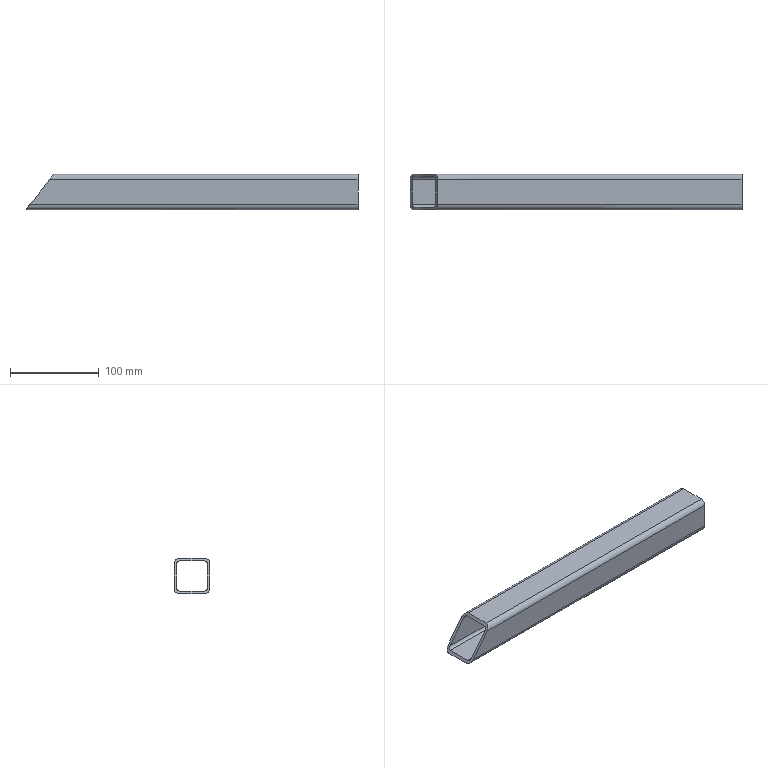Part | STEP file | right body front baffle fixing piece 2 | 1 solid | 18 faces | box 373.425 x 40 x 40 mm | volume 150546 mm3 | plane 10 | cylinder 8 | commonest cylinder face diameters 6 x4 12 x4